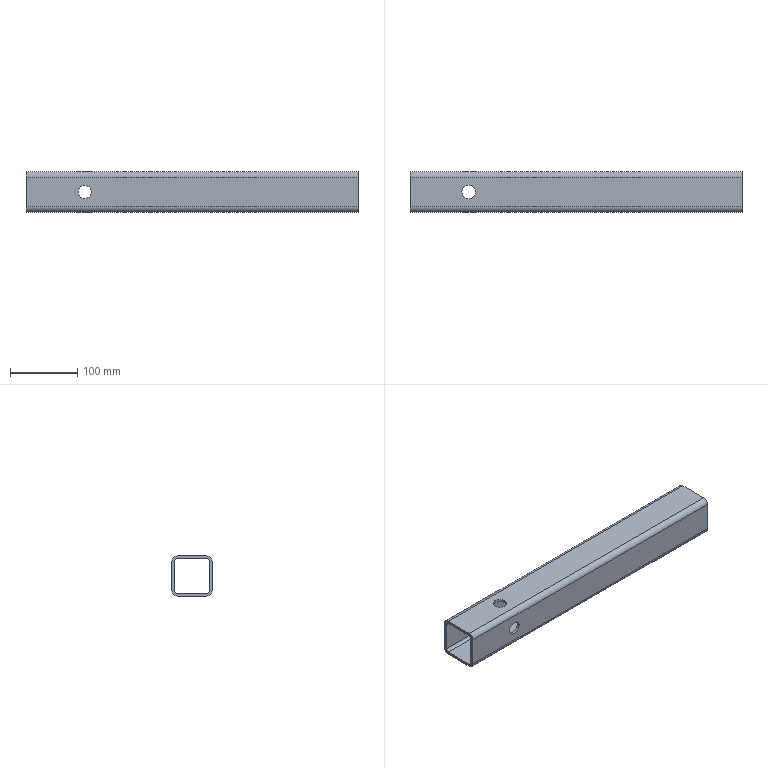Part | SolidWorks | features Cut 2, WeldMemberFeat 1, WeldmentFeature 1 | 1 solid | 26 faces | box 495 x 60 x 60 mm | volume 418098 mm3 | cylinder 16 | plane 10 | commonest cylinder face diameters 20 x8 8 x4 16 x4
STEP:
#1=CARTESIAN_POINT('',(-160.,-30.,10.));
#2=VERTEX_POINT('',#1);
#3=CARTESIAN_POINT('',(-160.,-30.,-10.));
#4=VERTEX_POINT('',#3);
#5=CARTESIAN_POINT('',(-160.,-30.,0.));
#6=DIRECTION('',(0.,-1.,0.));
#7=DIRECTION('',(-1.,0.,0.));
#8=AXIS2_PLACEMENT_3D('',#5,#6,#7);
#9=CIRCLE('',#8,10.);
#10=EDGE_CURVE('',#2,#4,#9,.T.);
#11=ORIENTED_EDGE('',*,*,#10,.T.);
#12=CARTESIAN_POINT('',(-160.,-26.,-10.));
#13=VERTEX_POINT('',#12);
#14=CARTESIAN_POINT('',(-160.,-58.284,-10.));
#15=DIRECTION('',(0.,1.,0.));
#16=VECTOR('',#15,1000.);
#17=LINE('',#14,#16);
#18=EDGE_CURVE('',#4,#13,#17,.T.);
#19=ORIENTED_EDGE('',*,*,#18,.T.);
#20=CARTESIAN_POINT('',(-160.,-26.,10.));
#21=VERTEX_POINT('',#20);
#22=CARTESIAN_POINT('',(-160.,-26.,0.));
#23=DIRECTION('',(0.,1.,0.));
#24=DIRECTION('',(-1.,0.,0.));
#25=AXIS2_PLACEMENT_3D('',#22,#23,#24);
#26=CIRCLE('',#25,10.);
#27=EDGE_CURVE('',#13,#21,#26,.T.);
#28=ORIENTED_EDGE('',*,*,#27,.T.);
#29=CARTESIAN_POINT('',(-160.,-58.284,10.));
#30=DIRECTION('',(0.,1.,0.));
#31=VECTOR('',#30,1000.);
#32=LINE('',#29,#31);
#33=EDGE_CURVE('',#2,#21,#32,.T.);
#34=ORIENTED_EDGE('',*,*,#33,.F.);
#35=EDGE_LOOP('',(#11,#19,#28,#34));
#36=FACE_OUTER_BOUND('',#35,.T.);
#37=CARTESIAN_POINT('',(-160.,-58.284,0.));
#38=DIRECTION('',(0.,1.,0.));
#39=DIRECTION('',(0.,0.,1.));
#40=AXIS2_PLACEMENT_3D('',#37,#38,#39);
#41=CYLINDRICAL_SURFACE('',#40,10.);
#42=ADVANCED_FACE('',(#36),#41,.F.);
#43=CARTESIAN_POINT('',(-160.,26.,10.));
#44=VERTEX_POINT('',#43);
#45=CARTESIAN_POINT('',(-160.,26.,-10.));
#46=VERTEX_POINT('',#45);
#47=CARTESIAN_POINT('',(-160.,26.,0.));
#48=DIRECTION('',(0.,-1.,0.));
#49=DIRECTION('',(1.,0.,0.));
#50=AXIS2_PLACEMENT_3D('',#47,#48,#49);
#51=CIRCLE('',#50,10.);
#52=EDGE_CURVE('',#44,#46,#51,.T.);
#53=ORIENTED_EDGE('',*,*,#52,.T.);
#54=CARTESIAN_POINT('',(-160.,30.,-10.));
#55=VERTEX_POINT('',#54);
#56=CARTESIAN_POINT('',(-160.,-58.284,-10.));
#57=DIRECTION('',(0.,1.,0.));
#58=VECTOR('',#57,1000.);
#59=LINE('',#56,#58);
#60=EDGE_CURVE('',#46,#55,#59,.T.);
#61=ORIENTED_EDGE('',*,*,#60,.T.);
#62=CARTESIAN_POINT('',(-160.,30.,10.));
#63=VERTEX_POINT('',#62);
#64=CARTESIAN_POINT('',(-160.,30.,0.));
#65=DIRECTION('',(0.,1.,0.));
#66=DIRECTION('',(0.,0.,1.));
#67=AXIS2_PLACEMENT_3D('',#64,#65,#66);
#68=CIRCLE('',#67,10.);
#69=EDGE_CURVE('',#55,#63,#68,.T.);
#70=ORIENTED_EDGE('',*,*,#69,.T.);
#71=CARTESIAN_POINT('',(-160.,-58.284,10.));
#72=DIRECTION('',(0.,1.,0.));
#73=VECTOR('',#72,1000.);
#74=LINE('',#71,#73);
#75=EDGE_CURVE('',#44,#63,#74,.T.);
#76=ORIENTED_EDGE('',*,*,#75,.F.);
#77=EDGE_LOOP('',(#53,#61,#70,#76));
#78=FACE_OUTER_BOUND('',#77,.T.);
#79=CARTESIAN_POINT('',(-160.,-58.284,0.));
#80=DIRECTION('',(0.,1.,0.));
#81=DIRECTION('',(0.,0.,1.));
#82=AXIS2_PLACEMENT_3D('',#79,#80,#81);
#83=CYLINDRICAL_SURFACE('',#82,10.);
#84=ADVANCED_FACE('',(#78),#83,.F.);
#85=CARTESIAN_POINT('',(-150.,0.,26.));
#86=VERTEX_POINT('',#85);
#87=CARTESIAN_POINT('',(-170.,0.,26.));
#88=VERTEX_POINT('',#87);
#89=CARTESIAN_POINT('',(-160.,0.,26.));
#90=DIRECTION('',(0.,0.,-1.));
#91=DIRECTION('',(-1.,0.,0.));
#92=AXIS2_PLACEMENT_3D('',#89,#90,#91);
#93=CIRCLE('',#92,10.);
#94=EDGE_CURVE('',#86,#88,#93,.T.);
#95=ORIENTED_EDGE('',*,*,#94,.T.);
#96=CARTESIAN_POINT('',(-170.,0.,30.));
#97=VERTEX_POINT('',#96);
#98=CARTESIAN_POINT('',(-170.,0.,-58.284));
#99=DIRECTION('',(0.,0.,1.));
#100=VECTOR('',#99,1000.);
#101=LINE('',#98,#100);
#102=EDGE_CURVE('',#88,#97,#101,.T.);
#103=ORIENTED_EDGE('',*,*,#102,.T.);
#104=CARTESIAN_POINT('',(-150.,0.,30.));
#105=VERTEX_POINT('',#104);
#106=CARTESIAN_POINT('',(-160.,0.,30.));
#107=DIRECTION('',(0.,0.,1.));
#108=DIRECTION('',(1.,0.,0.));
#109=AXIS2_PLACEMENT_3D('',#106,#107,#108);
#110=CIRCLE('',#109,10.);
#111=EDGE_CURVE('',#97,#105,#110,.T.);
#112=ORIENTED_EDGE('',*,*,#111,.T.);
#113=CARTESIAN_POINT('',(-150.,0.,-58.284));
#114=DIRECTION('',(0.,0.,1.));
#115=VECTOR('',#114,1000.);
#116=LINE('',#113,#115);
#117=EDGE_CURVE('',#86,#105,#116,.T.);
#118=ORIENTED_EDGE('',*,*,#117,.F.);
#119=EDGE_LOOP('',(#95,#103,#112,#118));
#120=FACE_OUTER_BOUND('',#119,.T.);
#121=CARTESIAN_POINT('',(-160.,0.,-58.284));
#122=DIRECTION('',(0.,0.,1.));
#123=DIRECTION('',(1.,0.,0.));
#124=AXIS2_PLACEMENT_3D('',#121,#122,#123);
#125=CYLINDRICAL_SURFACE('',#124,10.);
#126=ADVANCED_FACE('',(#120),#125,.F.);
#127=CARTESIAN_POINT('',(-150.,0.,-30.));
#128=VERTEX_POINT('',#127);
#129=CARTESIAN_POINT('',(-170.,0.,-30.));
#130=VERTEX_POINT('',#129);
#131=CARTESIAN_POINT('',(-160.,0.,-30.));
#132=DIRECTION('',(0.,0.,-1.));
#133=DIRECTION('',(1.,0.,0.));
#134=AXIS2_PLACEMENT_3D('',#131,#132,#133);
#135=CIRCLE('',#134,10.);
#136=EDGE_CURVE('',#128,#130,#135,.T.);
#137=ORIENTED_EDGE('',*,*,#136,.T.);
#138=CARTESIAN_POINT('',(-170.,0.,-26.));
#139=VERTEX_POINT('',#138);
#140=CARTESIAN_POINT('',(-170.,0.,-58.284));
#141=DIRECTION('',(0.,0.,1.));
#142=VECTOR('',#141,1000.);
#143=LINE('',#140,#142);
#144=EDGE_CURVE('',#130,#139,#143,.T.);
#145=ORIENTED_EDGE('',*,*,#144,.T.);
#146=CARTESIAN_POINT('',(-150.,0.,-26.));
#147=VERTEX_POINT('',#146);
#148=CARTESIAN_POINT('',(-160.,0.,-26.));
#149=DIRECTION('',(0.,0.,1.));
#150=DIRECTION('',(1.,0.,0.));
#151=AXIS2_PLACEMENT_3D('',#148,#149,#150);
#152=CIRCLE('',#151,10.);
#153=EDGE_CURVE('',#139,#147,#152,.T.);
#154=ORIENTED_EDGE('',*,*,#153,.T.);
#155=CARTESIAN_POINT('',(-150.,0.,-58.284));
#156=DIRECTION('',(0.,0.,1.));
#157=VECTOR('',#156,1000.);
#158=LINE('',#155,#157);
#159=EDGE_CURVE('',#128,#147,#158,.T.);
#160=ORIENTED_EDGE('',*,*,#159,.F.);
#161=EDGE_LOOP('',(#137,#145,#154,#160));
#162=FACE_OUTER_BOUND('',#161,.T.);
#163=CARTESIAN_POINT('',(-160.,0.,-58.284));
#164=DIRECTION('',(0.,0.,1.));
#165=DIRECTION('',(1.,0.,0.));
#166=AXIS2_PLACEMENT_3D('',#163,#164,#165);
#167=CYLINDRICAL_SURFACE('',#166,10.);
#168=ADVANCED_FACE('',(#162),#167,.F.);
#169=CARTESIAN_POINT('',(-247.5,30.,22.));
#170=VERTEX_POINT('',#169);
#171=CARTESIAN_POINT('',(-247.5,22.,30.));
#172=VERTEX_POINT('',#171);
#173=CARTESIAN_POINT('',(-247.5,22.,22.));
#174=DIRECTION('',(1.,0.,0.));
#175=DIRECTION('',(0.,1.,0.));
#176=AXIS2_PLACEMENT_3D('',#173,#174,#175);
#177=CIRCLE('',#176,8.);
#178=EDGE_CURVE('',#170,#172,#177,.T.);
#179=ORIENTED_EDGE('',*,*,#178,.T.);
#180=CARTESIAN_POINT('',(247.5,22.,30.));
#181=VERTEX_POINT('',#180);
#182=CARTESIAN_POINT('',(247.5,22.,30.));
#183=DIRECTION('',(-1.,0.,0.));
#184=VECTOR('',#183,1000.);
#185=LINE('',#182,#184);
#186=EDGE_CURVE('',#181,#172,#185,.T.);
#187=ORIENTED_EDGE('',*,*,#186,.F.);
#188=CARTESIAN_POINT('',(247.5,30.,22.));
#189=VERTEX_POINT('',#188);
#190=CARTESIAN_POINT('',(247.5,22.,22.));
#191=DIRECTION('',(1.,0.,0.));
#192=DIRECTION('',(0.,1.,0.));
#193=AXIS2_PLACEMENT_3D('',#190,#191,#192);
#194=CIRCLE('',#193,8.);
#195=EDGE_CURVE('',#189,#181,#194,.T.);
#196=ORIENTED_EDGE('',*,*,#195,.F.);
#197=CARTESIAN_POINT('',(247.5,30.,22.));
#198=DIRECTION('',(-1.,0.,0.));
#199=VECTOR('',#198,1000.);
#200=LINE('',#197,#199);
#201=EDGE_CURVE('',#189,#170,#200,.T.);
#202=ORIENTED_EDGE('',*,*,#201,.T.);
#203=EDGE_LOOP('',(#179,#187,#196,#202));
#204=FACE_OUTER_BOUND('',#203,.T.);
#205=CARTESIAN_POINT('',(247.5,22.,22.));
#206=DIRECTION('',(-1.,0.,0.));
#207=DIRECTION('',(0.,-1.,0.));
#208=AXIS2_PLACEMENT_3D('',#205,#206,#207);
#209=CYLINDRICAL_SURFACE('',#208,8.);
#210=ADVANCED_FACE('',(#204),#209,.T.);
#211=CARTESIAN_POINT('',(-160.,0.,30.));
#212=DIRECTION('',(0.,0.,1.));
#213=DIRECTION('',(1.,0.,0.));
#214=AXIS2_PLACEMENT_3D('',#211,#212,#213);
#215=CIRCLE('',#214,10.);
#216=EDGE_CURVE('',#105,#97,#215,.T.);
#217=ORIENTED_EDGE('',*,*,#216,.F.);
#218=ORIENTED_EDGE('',*,*,#111,.F.);
#219=EDGE_LOOP('',(#217,#218));
#220=FACE_BOUND('',#219,.T.);
#221=CARTESIAN_POINT('',(-247.5,-22.,30.));
#222=VERTEX_POINT('',#221);
#223=CARTESIAN_POINT('',(-247.5,22.,30.));
#224=DIRECTION('',(0.,-1.,0.));
#225=VECTOR('',#224,1000.);
#226=LINE('',#223,#225);
#227=EDGE_CURVE('',#172,#222,#226,.T.);
#228=ORIENTED_EDGE('',*,*,#227,.T.);
#229=CARTESIAN_POINT('',(247.5,-22.,30.));
#230=VERTEX_POINT('',#229);
#231=CARTESIAN_POINT('',(247.5,-22.,30.));
#232=DIRECTION('',(-1.,0.,0.));
#233=VECTOR('',#232,1000.);
#234=LINE('',#231,#233);
#235=EDGE_CURVE('',#230,#222,#234,.T.);
#236=ORIENTED_EDGE('',*,*,#235,.F.);
#237=CARTESIAN_POINT('',(247.5,22.,30.));
#238=DIRECTION('',(0.,-1.,0.));
#239=VECTOR('',#238,1000.);
#240=LINE('',#237,#239);
#241=EDGE_CURVE('',#181,#230,#240,.T.);
#242=ORIENTED_EDGE('',*,*,#241,.F.);
#243=ORIENTED_EDGE('',*,*,#186,.T.);
#244=EDGE_LOOP('',(#228,#236,#242,#243));
#245=FACE_OUTER_BOUND('',#244,.T.);
#246=CARTESIAN_POINT('',(247.5,22.,30.));
#247=DIRECTION('',(0.,0.,-1.));
#248=DIRECTION('',(-1.,0.,0.));
#249=AXIS2_PLACEMENT_3D('',#246,#247,#248);
#250=PLANE('',#249);
#251=ADVANCED_FACE('',(#220,#245),#250,.F.);
#252=CARTESIAN_POINT('',(-247.5,-30.,22.));
#253=VERTEX_POINT('',#252);
#254=CARTESIAN_POINT('',(-247.5,-22.,22.));
#255=DIRECTION('',(1.,0.,0.));
#256=DIRECTION('',(0.,1.,0.));
#257=AXIS2_PLACEMENT_3D('',#254,#255,#256);
#258=CIRCLE('',#257,8.);
#259=EDGE_CURVE('',#222,#253,#258,.T.);
#260=ORIENTED_EDGE('',*,*,#259,.T.);
#261=CARTESIAN_POINT('',(247.5,-30.,22.));
#262=VERTEX_POINT('',#261);
#263=CARTESIAN_POINT('',(247.5,-30.,22.));
#264=DIRECTION('',(-1.,0.,0.));
#265=VECTOR('',#264,1000.);
#266=LINE('',#263,#265);
#267=EDGE_CURVE('',#262,#253,#266,.T.);
#268=ORIENTED_EDGE('',*,*,#267,.F.);
#269=CARTESIAN_POINT('',(247.5,-22.,22.));
#270=DIRECTION('',(1.,0.,0.));
#271=DIRECTION('',(0.,1.,0.));
#272=AXIS2_PLACEMENT_3D('',#269,#270,#271);
#273=CIRCLE('',#272,8.);
#274=EDGE_CURVE('',#230,#262,#273,.T.);
#275=ORIENTED_EDGE('',*,*,#274,.F.);
#276=ORIENTED_EDGE('',*,*,#235,.T.);
#277=EDGE_LOOP('',(#260,#268,#275,#276));
#278=FACE_OUTER_BOUND('',#277,.T.);
#279=CARTESIAN_POINT('',(247.5,-22.,22.));
#280=DIRECTION('',(-1.,0.,0.));
#281=DIRECTION('',(0.,-1.,0.));
#282=AXIS2_PLACEMENT_3D('',#279,#280,#281);
#283=CYLINDRICAL_SURFACE('',#282,8.);
#284=ADVANCED_FACE('',(#278),#283,.T.);
#285=ORIENTED_EDGE('',*,*,#10,.F.);
#286=CARTESIAN_POINT('',(-160.,-30.,0.));
#287=DIRECTION('',(0.,-1.,0.));
#288=DIRECTION('',(-1.,0.,0.));
#289=AXIS2_PLACEMENT_3D('',#286,#287,#288);
#290=CIRCLE('',#289,10.);
#291=EDGE_CURVE('',#4,#2,#290,.T.);
#292=ORIENTED_EDGE('',*,*,#291,.F.);
#293=EDGE_LOOP('',(#285,#292));
#294=FACE_BOUND('',#293,.T.);
#295=CARTESIAN_POINT('',(-247.5,-30.,-22.));
#296=VERTEX_POINT('',#295);
#297=CARTESIAN_POINT('',(-247.5,-30.,-22.));
#298=DIRECTION('',(0.,0.,-1.));
#299=VECTOR('',#298,1000.);
#300=LINE('',#297,#299);
#301=EDGE_CURVE('',#253,#296,#300,.T.);
#302=ORIENTED_EDGE('',*,*,#301,.T.);
#303=CARTESIAN_POINT('',(247.5,-30.,-22.));
#304=VERTEX_POINT('',#303);
#305=CARTESIAN_POINT('',(247.5,-30.,-22.));
#306=DIRECTION('',(-1.,0.,0.));
#307=VECTOR('',#306,1000.);
#308=LINE('',#305,#307);
#309=EDGE_CURVE('',#304,#296,#308,.T.);
#310=ORIENTED_EDGE('',*,*,#309,.F.);
#311=CARTESIAN_POINT('',(247.5,-30.,-22.));
#312=DIRECTION('',(0.,0.,-1.));
#313=VECTOR('',#312,1000.);
#314=LINE('',#311,#313);
#315=EDGE_CURVE('',#262,#304,#314,.T.);
#316=ORIENTED_EDGE('',*,*,#315,.F.);
#317=ORIENTED_EDGE('',*,*,#267,.T.);
#318=EDGE_LOOP('',(#302,#310,#316,#317));
#319=FACE_OUTER_BOUND('',#318,.T.);
#320=CARTESIAN_POINT('',(247.5,-30.,-22.));
#321=DIRECTION('',(0.,1.,0.));
#322=DIRECTION('',(-1.,0.,0.));
#323=AXIS2_PLACEMENT_3D('',#320,#321,#322);
#324=PLANE('',#323);
#325=ADVANCED_FACE('',(#294,#319),#324,.F.);
#326=CARTESIAN_POINT('',(-247.5,-22.,-30.));
#327=VERTEX_POINT('',#326);
#328=CARTESIAN_POINT('',(-247.5,-22.,-22.));
#329=DIRECTION('',(1.,0.,0.));
#330=DIRECTION('',(0.,1.,0.));
#331=AXIS2_PLACEMENT_3D('',#328,#329,#330);
#332=CIRCLE('',#331,8.);
#333=EDGE_CURVE('',#296,#327,#332,.T.);
#334=ORIENTED_EDGE('',*,*,#333,.T.);
#335=CARTESIAN_POINT('',(247.5,-22.,-30.));
#336=VERTEX_POINT('',#335);
#337=CARTESIAN_POINT('',(247.5,-22.,-30.));
#338=DIRECTION('',(-1.,0.,0.));
#339=VECTOR('',#338,1000.);
#340=LINE('',#337,#339);
#341=EDGE_CURVE('',#336,#327,#340,.T.);
#342=ORIENTED_EDGE('',*,*,#341,.F.);
#343=CARTESIAN_POINT('',(247.5,-22.,-22.));
#344=DIRECTION('',(1.,0.,0.));
#345=DIRECTION('',(0.,1.,0.));
#346=AXIS2_PLACEMENT_3D('',#343,#344,#345);
#347=CIRCLE('',#346,8.);
#348=EDGE_CURVE('',#304,#336,#347,.T.);
#349=ORIENTED_EDGE('',*,*,#348,.F.);
#350=ORIENTED_EDGE('',*,*,#309,.T.);
#351=EDGE_LOOP('',(#334,#342,#349,#350));
#352=FACE_OUTER_BOUND('',#351,.T.);
#353=CARTESIAN_POINT('',(247.5,-22.,-22.));
#354=DIRECTION('',(-1.,0.,0.));
#355=DIRECTION('',(0.,-1.,0.));
#356=AXIS2_PLACEMENT_3D('',#353,#354,#355);
#357=CYLINDRICAL_SURFACE('',#356,8.);
#358=ADVANCED_FACE('',(#352),#357,.T.);
#359=ORIENTED_EDGE('',*,*,#136,.F.);
#360=CARTESIAN_POINT('',(-160.,0.,-30.));
#361=DIRECTION('',(0.,0.,-1.));
#362=DIRECTION('',(1.,0.,0.));
#363=AXIS2_PLACEMENT_3D('',#360,#361,#362);
#364=CIRCLE('',#363,10.);
#365=EDGE_CURVE('',#130,#128,#364,.T.);
#366=ORIENTED_EDGE('',*,*,#365,.F.);
#367=EDGE_LOOP('',(#359,#366));
#368=FACE_BOUND('',#367,.T.);
#369=CARTESIAN_POINT('',(-247.5,22.,-30.));
#370=VERTEX_POINT('',#369);
#371=CARTESIAN_POINT('',(-247.5,-22.,-30.));
#372=DIRECTION('',(0.,1.,0.));
#373=VECTOR('',#372,1000.);
#374=LINE('',#371,#373);
#375=EDGE_CURVE('',#327,#370,#374,.T.);
#376=ORIENTED_EDGE('',*,*,#375,.T.);
#377=CARTESIAN_POINT('',(247.5,22.,-30.));
#378=VERTEX_POINT('',#377);
#379=CARTESIAN_POINT('',(247.5,22.,-30.));
#380=DIRECTION('',(-1.,0.,0.));
#381=VECTOR('',#380,1000.);
#382=LINE('',#379,#381);
#383=EDGE_CURVE('',#378,#370,#382,.T.);
#384=ORIENTED_EDGE('',*,*,#383,.F.);
#385=CARTESIAN_POINT('',(247.5,-22.,-30.));
#386=DIRECTION('',(0.,1.,0.));
#387=VECTOR('',#386,1000.);
#388=LINE('',#385,#387);
#389=EDGE_CURVE('',#336,#378,#388,.T.);
#390=ORIENTED_EDGE('',*,*,#389,.F.);
#391=ORIENTED_EDGE('',*,*,#341,.T.);
#392=EDGE_LOOP('',(#376,#384,#390,#391));
#393=FACE_OUTER_BOUND('',#392,.T.);
#394=CARTESIAN_POINT('',(247.5,-22.,-30.));
#395=DIRECTION('',(0.,0.,1.));
#396=DIRECTION('',(1.,0.,0.));
#397=AXIS2_PLACEMENT_3D('',#394,#395,#396);
#398=PLANE('',#397);
#399=ADVANCED_FACE('',(#368,#393),#398,.F.);
#400=CARTESIAN_POINT('',(-247.5,30.,-22.));
#401=VERTEX_POINT('',#400);
#402=CARTESIAN_POINT('',(-247.5,22.,-22.));
#403=DIRECTION('',(1.,0.,0.));
#404=DIRECTION('',(0.,1.,0.));
#405=AXIS2_PLACEMENT_3D('',#402,#403,#404);
#406=CIRCLE('',#405,8.);
#407=EDGE_CURVE('',#370,#401,#406,.T.);
#408=ORIENTED_EDGE('',*,*,#407,.T.);
#409=CARTESIAN_POINT('',(247.5,30.,-22.));
#410=VERTEX_POINT('',#409);
#411=CARTESIAN_POINT('',(247.5,30.,-22.));
#412=DIRECTION('',(-1.,0.,0.));
#413=VECTOR('',#412,1000.);
#414=LINE('',#411,#413);
#415=EDGE_CURVE('',#410,#401,#414,.T.);
#416=ORIENTED_EDGE('',*,*,#415,.F.);
#417=CARTESIAN_POINT('',(247.5,22.,-22.));
#418=DIRECTION('',(1.,0.,0.));
#419=DIRECTION('',(0.,1.,0.));
#420=AXIS2_PLACEMENT_3D('',#417,#418,#419);
#421=CIRCLE('',#420,8.);
#422=EDGE_CURVE('',#378,#410,#421,.T.);
#423=ORIENTED_EDGE('',*,*,#422,.F.);
#424=ORIENTED_EDGE('',*,*,#383,.T.);
#425=EDGE_LOOP('',(#408,#416,#423,#424));
#426=FACE_OUTER_BOUND('',#425,.T.);
#427=CARTESIAN_POINT('',(247.5,22.,-22.));
#428=DIRECTION('',(-1.,0.,0.));
#429=DIRECTION('',(0.,-1.,0.));
#430=AXIS2_PLACEMENT_3D('',#427,#428,#429);
#431=CYLINDRICAL_SURFACE('',#430,8.);
#432=ADVANCED_FACE('',(#426),#431,.T.);
#433=CARTESIAN_POINT('',(-247.5,-22.,26.));
#434=VERTEX_POINT('',#433);
#435=CARTESIAN_POINT('',(-247.5,-26.,22.));
#436=VERTEX_POINT('',#435);
#437=CARTESIAN_POINT('',(-247.5,-22.,22.));
#438=DIRECTION('',(1.,0.,0.));
#439=DIRECTION('',(0.,1.,0.));
#440=AXIS2_PLACEMENT_3D('',#437,#438,#439);
#441=CIRCLE('',#440,4.);
#442=EDGE_CURVE('',#434,#436,#441,.T.);
#443=ORIENTED_EDGE('',*,*,#442,.F.);
#444=CARTESIAN_POINT('',(247.5,-22.,26.));
#445=VERTEX_POINT('',#444);
#446=CARTESIAN_POINT('',(247.5,-22.,26.));
#447=DIRECTION('',(-1.,0.,0.));
#448=VECTOR('',#447,1000.);
#449=LINE('',#446,#448);
#450=EDGE_CURVE('',#445,#434,#449,.T.);
#451=ORIENTED_EDGE('',*,*,#450,.F.);
#452=CARTESIAN_POINT('',(247.5,-26.,22.));
#453=VERTEX_POINT('',#452);
#454=CARTESIAN_POINT('',(247.5,-22.,22.));
#455=DIRECTION('',(1.,0.,0.));
#456=DIRECTION('',(0.,1.,0.));
#457=AXIS2_PLACEMENT_3D('',#454,#455,#456);
#458=CIRCLE('',#457,4.);
#459=EDGE_CURVE('',#445,#453,#458,.T.);
#460=ORIENTED_EDGE('',*,*,#459,.T.);
#461=CARTESIAN_POINT('',(247.5,-26.,22.));
#462=DIRECTION('',(-1.,0.,0.));
#463=VECTOR('',#462,1000.);
#464=LINE('',#461,#463);
#465=EDGE_CURVE('',#453,#436,#464,.T.);
#466=ORIENTED_EDGE('',*,*,#465,.T.);
#467=EDGE_LOOP('',(#443,#451,#460,#466));
#468=FACE_OUTER_BOUND('',#467,.T.);
#469=CARTESIAN_POINT('',(247.5,-22.,22.));
#470=DIRECTION('',(-1.,0.,0.));
#471=DIRECTION('',(0.,-1.,0.));
#472=AXIS2_PLACEMENT_3D('',#469,#470,#471);
#473=CYLINDRICAL_SURFACE('',#472,4.);
#474=ADVANCED_FACE('',(#468),#473,.F.);
#475=ORIENTED_EDGE('',*,*,#94,.F.);
#476=CARTESIAN_POINT('',(-160.,0.,26.));
#477=DIRECTION('',(0.,0.,-1.));
#478=DIRECTION('',(-1.,0.,0.));
#479=AXIS2_PLACEMENT_3D('',#476,#477,#478);
#480=CIRCLE('',#479,10.);
#481=EDGE_CURVE('',#88,#86,#480,.T.);
#482=ORIENTED_EDGE('',*,*,#481,.F.);
#483=EDGE_LOOP('',(#475,#482));
#484=FACE_BOUND('',#483,.T.);
#485=CARTESIAN_POINT('',(-247.5,22.,26.));
#486=VERTEX_POINT('',#485);
#487=CARTESIAN_POINT('',(-247.5,22.,26.));
#488=DIRECTION('',(0.,-1.,0.));
#489=VECTOR('',#488,1000.);
#490=LINE('',#487,#489);
#491=EDGE_CURVE('',#486,#434,#490,.T.);
#492=ORIENTED_EDGE('',*,*,#491,.F.);
#493=CARTESIAN_POINT('',(247.5,22.,26.));
#494=VERTEX_POINT('',#493);
#495=CARTESIAN_POINT('',(247.5,22.,26.));
#496=DIRECTION('',(-1.,0.,0.));
#497=VECTOR('',#496,1000.);
#498=LINE('',#495,#497);
#499=EDGE_CURVE('',#494,#486,#498,.T.);
#500=ORIENTED_EDGE('',*,*,#499,.F.);
#501=CARTESIAN_POINT('',(247.5,22.,26.));
#502=DIRECTION('',(0.,-1.,0.));
#503=VECTOR('',#502,1000.);
#504=LINE('',#501,#503);
#505=EDGE_CURVE('',#494,#445,#504,.T.);
#506=ORIENTED_EDGE('',*,*,#505,.T.);
#507=ORIENTED_EDGE('',*,*,#450,.T.);
#508=EDGE_LOOP('',(#492,#500,#506,#507));
#509=FACE_OUTER_BOUND('',#508,.T.);
#510=CARTESIAN_POINT('',(247.5,22.,26.));
#511=DIRECTION('',(0.,0.,-1.));
#512=DIRECTION('',(-1.,0.,0.));
#513=AXIS2_PLACEMENT_3D('',#510,#511,#512);
#514=PLANE('',#513);
#515=ADVANCED_FACE('',(#484,#509),#514,.T.);
#516=CARTESIAN_POINT('',(-247.5,26.,22.));
#517=VERTEX_POINT('',#516);
#518=CARTESIAN_POINT('',(-247.5,22.,22.));
#519=DIRECTION('',(1.,0.,0.));
#520=DIRECTION('',(0.,1.,0.));
#521=AXIS2_PLACEMENT_3D('',#518,#519,#520);
#522=CIRCLE('',#521,4.);
#523=EDGE_CURVE('',#517,#486,#522,.T.);
#524=ORIENTED_EDGE('',*,*,#523,.F.);
#525=CARTESIAN_POINT('',(247.5,26.,22.));
#526=VERTEX_POINT('',#525);
#527=CARTESIAN_POINT('',(247.5,26.,22.));
#528=DIRECTION('',(-1.,0.,0.));
#529=VECTOR('',#528,1000.);
#530=LINE('',#527,#529);
#531=EDGE_CURVE('',#526,#517,#530,.T.);
#532=ORIENTED_EDGE('',*,*,#531,.F.);
#533=CARTESIAN_POINT('',(247.5,22.,22.));
#534=DIRECTION('',(1.,0.,0.));
#535=DIRECTION('',(0.,1.,0.));
#536=AXIS2_PLACEMENT_3D('',#533,#534,#535);
#537=CIRCLE('',#536,4.);
#538=EDGE_CURVE('',#526,#494,#537,.T.);
#539=ORIENTED_EDGE('',*,*,#538,.T.);
#540=ORIENTED_EDGE('',*,*,#499,.T.);
#541=EDGE_LOOP('',(#524,#532,#539,#540));
#542=FACE_OUTER_BOUND('',#541,.T.);
#543=CARTESIAN_POINT('',(247.5,22.,22.));
#544=DIRECTION('',(-1.,0.,0.));
#545=DIRECTION('',(0.,-1.,0.));
#546=AXIS2_PLACEMENT_3D('',#543,#544,#545);
#547=CYLINDRICAL_SURFACE('',#546,4.);
#548=ADVANCED_FACE('',(#542),#547,.F.);
#549=ORIENTED_EDGE('',*,*,#52,.F.);
#550=CARTESIAN_POINT('',(-160.,26.,0.));
#551=DIRECTION('',(0.,-1.,0.));
#552=DIRECTION('',(1.,0.,0.));
#553=AXIS2_PLACEMENT_3D('',#550,#551,#552);
#554=CIRCLE('',#553,10.);
#555=EDGE_CURVE('',#46,#44,#554,.T.);
#556=ORIENTED_EDGE('',*,*,#555,.F.);
#557=EDGE_LOOP('',(#549,#556));
#558=FACE_BOUND('',#557,.T.);
#559=CARTESIAN_POINT('',(-247.5,26.,-22.));
#560=VERTEX_POINT('',#559);
#561=CARTESIAN_POINT('',(-247.5,26.,22.));
#562=DIRECTION('',(0.,0.,1.));
#563=VECTOR('',#562,1000.);
#564=LINE('',#561,#563);
#565=EDGE_CURVE('',#560,#517,#564,.T.);
#566=ORIENTED_EDGE('',*,*,#565,.F.);
#567=CARTESIAN_POINT('',(247.5,26.,-22.));
#568=VERTEX_POINT('',#567);
#569=CARTESIAN_POINT('',(247.5,26.,-22.));
#570=DIRECTION('',(-1.,0.,0.));
#571=VECTOR('',#570,1000.);
#572=LINE('',#569,#571);
#573=EDGE_CURVE('',#568,#560,#572,.T.);
#574=ORIENTED_EDGE('',*,*,#573,.F.);
#575=CARTESIAN_POINT('',(247.5,26.,22.));
#576=DIRECTION('',(0.,0.,1.));
#577=VECTOR('',#576,1000.);
#578=LINE('',#575,#577);
#579=EDGE_CURVE('',#568,#526,#578,.T.);
#580=ORIENTED_EDGE('',*,*,#579,.T.);
#581=ORIENTED_EDGE('',*,*,#531,.T.);
#582=EDGE_LOOP('',(#566,#574,#580,#581));
#583=FACE_OUTER_BOUND('',#582,.T.);
#584=CARTESIAN_POINT('',(247.5,26.,22.));
#585=DIRECTION('',(0.,-1.,0.));
#586=DIRECTION('',(1.,0.,0.));
#587=AXIS2_PLACEMENT_3D('',#584,#585,#586);
#588=PLANE('',#587);
#589=ADVANCED_FACE('',(#558,#583),#588,.T.);
#590=CARTESIAN_POINT('',(-247.5,22.,-26.));
#591=VERTEX_POINT('',#590);
#592=CARTESIAN_POINT('',(-247.5,22.,-22.));
#593=DIRECTION('',(1.,0.,0.));
#594=DIRECTION('',(0.,1.,0.));
#595=AXIS2_PLACEMENT_3D('',#592,#593,#594);
#596=CIRCLE('',#595,4.);
#597=EDGE_CURVE('',#591,#560,#596,.T.);
#598=ORIENTED_EDGE('',*,*,#597,.F.);
#599=CARTESIAN_POINT('',(247.5,22.,-26.));
#600=VERTEX_POINT('',#599);
#601=CARTESIAN_POINT('',(247.5,22.,-26.));
#602=DIRECTION('',(-1.,0.,0.));
#603=VECTOR('',#602,1000.);
#604=LINE('',#601,#603);
#605=EDGE_CURVE('',#600,#591,#604,.T.);
#606=ORIENTED_EDGE('',*,*,#605,.F.);
#607=CARTESIAN_POINT('',(247.5,22.,-22.));
#608=DIRECTION('',(1.,0.,0.));
#609=DIRECTION('',(0.,1.,0.));
#610=AXIS2_PLACEMENT_3D('',#607,#608,#609);
#611=CIRCLE('',#610,4.);
#612=EDGE_CURVE('',#600,#568,#611,.T.);
#613=ORIENTED_EDGE('',*,*,#612,.T.);
#614=ORIENTED_EDGE('',*,*,#573,.T.);
#615=EDGE_LOOP('',(#598,#606,#613,#614));
#616=FACE_OUTER_BOUND('',#615,.T.);
#617=CARTESIAN_POINT('',(247.5,22.,-22.));
#618=DIRECTION('',(-1.,0.,0.));
#619=DIRECTION('',(0.,-1.,0.));
#620=AXIS2_PLACEMENT_3D('',#617,#618,#619);
#621=CYLINDRICAL_SURFACE('',#620,4.);
#622=ADVANCED_FACE('',(#616),#621,.F.);
#623=CARTESIAN_POINT('',(-160.,0.,-26.));
#624=DIRECTION('',(0.,0.,1.));
#625=DIRECTION('',(1.,0.,0.));
#626=AXIS2_PLACEMENT_3D('',#623,#624,#625);
#627=CIRCLE('',#626,10.);
#628=EDGE_CURVE('',#147,#139,#627,.T.);
#629=ORIENTED_EDGE('',*,*,#628,.F.);
#630=ORIENTED_EDGE('',*,*,#153,.F.);
#631=EDGE_LOOP('',(#629,#630));
#632=FACE_BOUND('',#631,.T.);
#633=CARTESIAN_POINT('',(-247.5,-22.,-26.));
#634=VERTEX_POINT('',#633);
#635=CARTESIAN_POINT('',(-247.5,-22.,-26.));
#636=DIRECTION('',(0.,1.,0.));
#637=VECTOR('',#636,1000.);
#638=LINE('',#635,#637);
#639=EDGE_CURVE('',#634,#591,#638,.T.);
#640=ORIENTED_EDGE('',*,*,#639,.F.);
#641=CARTESIAN_POINT('',(247.5,-22.,-26.));
#642=VERTEX_POINT('',#641);
#643=CARTESIAN_POINT('',(247.5,-22.,-26.));
#644=DIRECTION('',(-1.,0.,0.));
#645=VECTOR('',#644,1000.);
#646=LINE('',#643,#645);
#647=EDGE_CURVE('',#642,#634,#646,.T.);
#648=ORIENTED_EDGE('',*,*,#647,.F.);
#649=CARTESIAN_POINT('',(247.5,-22.,-26.));
#650=DIRECTION('',(0.,1.,0.));
#651=VECTOR('',#650,1000.);
#652=LINE('',#649,#651);
#653=EDGE_CURVE('',#642,#600,#652,.T.);
#654=ORIENTED_EDGE('',*,*,#653,.T.);
#655=ORIENTED_EDGE('',*,*,#605,.T.);
#656=EDGE_LOOP('',(#640,#648,#654,#655));
#657=FACE_OUTER_BOUND('',#656,.T.);
#658=CARTESIAN_POINT('',(247.5,-22.,-26.));
#659=DIRECTION('',(0.,0.,1.));
#660=DIRECTION('',(1.,0.,0.));
#661=AXIS2_PLACEMENT_3D('',#658,#659,#660);
#662=PLANE('',#661);
#663=ADVANCED_FACE('',(#632,#657),#662,.T.);
#664=CARTESIAN_POINT('',(-247.5,-26.,-22.));
#665=VERTEX_POINT('',#664);
#666=CARTESIAN_POINT('',(-247.5,-22.,-22.));
#667=DIRECTION('',(1.,0.,0.));
#668=DIRECTION('',(0.,1.,0.));
#669=AXIS2_PLACEMENT_3D('',#666,#667,#668);
#670=CIRCLE('',#669,4.);
#671=EDGE_CURVE('',#665,#634,#670,.T.);
#672=ORIENTED_EDGE('',*,*,#671,.F.);
#673=CARTESIAN_POINT('',(247.5,-26.,-22.));
#674=VERTEX_POINT('',#673);
#675=CARTESIAN_POINT('',(247.5,-26.,-22.));
#676=DIRECTION('',(-1.,0.,0.));
#677=VECTOR('',#676,1000.);
#678=LINE('',#675,#677);
#679=EDGE_CURVE('',#674,#665,#678,.T.);
#680=ORIENTED_EDGE('',*,*,#679,.F.);
#681=CARTESIAN_POINT('',(247.5,-22.,-22.));
#682=DIRECTION('',(1.,0.,0.));
#683=DIRECTION('',(0.,1.,0.));
#684=AXIS2_PLACEMENT_3D('',#681,#682,#683);
#685=CIRCLE('',#684,4.);
#686=EDGE_CURVE('',#674,#642,#685,.T.);
#687=ORIENTED_EDGE('',*,*,#686,.T.);
#688=ORIENTED_EDGE('',*,*,#647,.T.);
#689=EDGE_LOOP('',(#672,#680,#687,#688));
#690=FACE_OUTER_BOUND('',#689,.T.);
#691=CARTESIAN_POINT('',(247.5,-22.,-22.));
#692=DIRECTION('',(-1.,0.,0.));
#693=DIRECTION('',(0.,-1.,0.));
#694=AXIS2_PLACEMENT_3D('',#691,#692,#693);
#695=CYLINDRICAL_SURFACE('',#694,4.);
#696=ADVANCED_FACE('',(#690),#695,.F.);
#697=CARTESIAN_POINT('',(-160.,-26.,0.));
#698=DIRECTION('',(0.,1.,0.));
#699=DIRECTION('',(-1.,0.,0.));
#700=AXIS2_PLACEMENT_3D('',#697,#698,#699);
#701=CIRCLE('',#700,10.);
#702=EDGE_CURVE('',#21,#13,#701,.T.);
#703=ORIENTED_EDGE('',*,*,#702,.F.);
#704=ORIENTED_EDGE('',*,*,#27,.F.);
#705=EDGE_LOOP('',(#703,#704));
#706=FACE_BOUND('',#705,.T.);
#707=CARTESIAN_POINT('',(-247.5,-26.,-22.));
#708=DIRECTION('',(0.,0.,-1.));
#709=VECTOR('',#708,1000.);
#710=LINE('',#707,#709);
#711=EDGE_CURVE('',#436,#665,#710,.T.);
#712=ORIENTED_EDGE('',*,*,#711,.F.);
#713=ORIENTED_EDGE('',*,*,#465,.F.);
#714=CARTESIAN_POINT('',(247.5,-26.,-22.));
#715=DIRECTION('',(0.,0.,-1.));
#716=VECTOR('',#715,1000.);
#717=LINE('',#714,#716);
#718=EDGE_CURVE('',#453,#674,#717,.T.);
#719=ORIENTED_EDGE('',*,*,#718,.T.);
#720=ORIENTED_EDGE('',*,*,#679,.T.);
#721=EDGE_LOOP('',(#712,#713,#719,#720));
#722=FACE_OUTER_BOUND('',#721,.T.);
#723=CARTESIAN_POINT('',(247.5,-26.,-22.));
#724=DIRECTION('',(0.,1.,0.));
#725=DIRECTION('',(-1.,0.,0.));
#726=AXIS2_PLACEMENT_3D('',#723,#724,#725);
#727=PLANE('',#726);
#728=ADVANCED_FACE('',(#706,#722),#727,.T.);
#729=CARTESIAN_POINT('',(-160.,30.,0.));
#730=DIRECTION('',(0.,1.,0.));
#731=DIRECTION('',(0.,0.,1.));
#732=AXIS2_PLACEMENT_3D('',#729,#730,#731);
#733=CIRCLE('',#732,10.);
#734=EDGE_CURVE('',#63,#55,#733,.T.);
#735=ORIENTED_EDGE('',*,*,#734,.F.);
#736=ORIENTED_EDGE('',*,*,#69,.F.);
#737=EDGE_LOOP('',(#735,#736));
#738=FACE_BOUND('',#737,.T.);
#739=CARTESIAN_POINT('',(-247.5,30.,22.));
#740=DIRECTION('',(0.,0.,1.));
#741=VECTOR('',#740,1000.);
#742=LINE('',#739,#741);
#743=EDGE_CURVE('',#401,#170,#742,.T.);
#744=ORIENTED_EDGE('',*,*,#743,.T.);
#745=ORIENTED_EDGE('',*,*,#201,.F.);
#746=CARTESIAN_POINT('',(247.5,30.,22.));
#747=DIRECTION('',(0.,0.,1.));
#748=VECTOR('',#747,1000.);
#749=LINE('',#746,#748);
#750=EDGE_CURVE('',#410,#189,#749,.T.);
#751=ORIENTED_EDGE('',*,*,#750,.F.);
#752=ORIENTED_EDGE('',*,*,#415,.T.);
#753=EDGE_LOOP('',(#744,#745,#751,#752));
#754=FACE_OUTER_BOUND('',#753,.T.);
#755=CARTESIAN_POINT('',(247.5,30.,22.));
#756=DIRECTION('',(0.,-1.,0.));
#757=DIRECTION('',(1.,0.,0.));
#758=AXIS2_PLACEMENT_3D('',#755,#756,#757);
#759=PLANE('',#758);
#760=ADVANCED_FACE('',(#738,#754),#759,.F.);
#761=ORIENTED_EDGE('',*,*,#459,.F.);
#762=ORIENTED_EDGE('',*,*,#505,.F.);
#763=ORIENTED_EDGE('',*,*,#538,.F.);
#764=ORIENTED_EDGE('',*,*,#579,.F.);
#765=ORIENTED_EDGE('',*,*,#612,.F.);
#766=ORIENTED_EDGE('',*,*,#653,.F.);
#767=ORIENTED_EDGE('',*,*,#686,.F.);
#768=ORIENTED_EDGE('',*,*,#718,.F.);
#769=EDGE_LOOP('',(#761,#762,#763,#764,#765,#766,#767,#768));
#770=FACE_BOUND('',#769,.T.);
#771=ORIENTED_EDGE('',*,*,#195,.T.);
#772=ORIENTED_EDGE('',*,*,#241,.T.);
#773=ORIENTED_EDGE('',*,*,#274,.T.);
#774=ORIENTED_EDGE('',*,*,#315,.T.);
#775=ORIENTED_EDGE('',*,*,#348,.T.);
#776=ORIENTED_EDGE('',*,*,#389,.T.);
#777=ORIENTED_EDGE('',*,*,#422,.T.);
#778=ORIENTED_EDGE('',*,*,#750,.T.);
#779=EDGE_LOOP('',(#771,#772,#773,#774,#775,#776,#777,#778));
#780=FACE_OUTER_BOUND('',#779,.T.);
#781=CARTESIAN_POINT('',(247.5,22.,22.));
#782=DIRECTION('',(1.,0.,0.));
#783=DIRECTION('',(0.,1.,0.));
#784=AXIS2_PLACEMENT_3D('',#781,#782,#783);
#785=PLANE('',#784);
#786=ADVANCED_FACE('',(#770,#780),#785,.T.);
#787=ORIENTED_EDGE('',*,*,#442,.T.);
#788=ORIENTED_EDGE('',*,*,#711,.T.);
#789=ORIENTED_EDGE('',*,*,#671,.T.);
#790=ORIENTED_EDGE('',*,*,#639,.T.);
#791=ORIENTED_EDGE('',*,*,#597,.T.);
#792=ORIENTED_EDGE('',*,*,#565,.T.);
#793=ORIENTED_EDGE('',*,*,#523,.T.);
#794=ORIENTED_EDGE('',*,*,#491,.T.);
#795=EDGE_LOOP('',(#787,#788,#789,#790,#791,#792,#793,#794));
#796=FACE_BOUND('',#795,.T.);
#797=ORIENTED_EDGE('',*,*,#178,.F.);
#798=ORIENTED_EDGE('',*,*,#743,.F.);
#799=ORIENTED_EDGE('',*,*,#407,.F.);
#800=ORIENTED_EDGE('',*,*,#375,.F.);
#801=ORIENTED_EDGE('',*,*,#333,.F.);
#802=ORIENTED_EDGE('',*,*,#301,.F.);
#803=ORIENTED_EDGE('',*,*,#259,.F.);
#804=ORIENTED_EDGE('',*,*,#227,.F.);
#805=EDGE_LOOP('',(#797,#798,#799,#800,#801,#802,#803,#804));
#806=FACE_OUTER_BOUND('',#805,.T.);
#807=CARTESIAN_POINT('',(-247.5,22.,22.));
#808=DIRECTION('',(1.,0.,0.));
#809=DIRECTION('',(0.,1.,0.));
#810=AXIS2_PLACEMENT_3D('',#807,#808,#809);
#811=PLANE('',#810);
#812=ADVANCED_FACE('',(#796,#806),#811,.F.);
#813=ORIENTED_EDGE('',*,*,#144,.F.);
#814=ORIENTED_EDGE('',*,*,#365,.T.);
#815=ORIENTED_EDGE('',*,*,#159,.T.);
#816=ORIENTED_EDGE('',*,*,#628,.T.);
#817=EDGE_LOOP('',(#813,#814,#815,#816));
#818=FACE_OUTER_BOUND('',#817,.T.);
#819=CARTESIAN_POINT('',(-160.,0.,-58.284));
#820=DIRECTION('',(0.,0.,1.));
#821=DIRECTION('',(1.,0.,0.));
#822=AXIS2_PLACEMENT_3D('',#819,#820,#821);
#823=CYLINDRICAL_SURFACE('',#822,10.);
#824=ADVANCED_FACE('',(#818),#823,.F.);
#825=ORIENTED_EDGE('',*,*,#102,.F.);
#826=ORIENTED_EDGE('',*,*,#481,.T.);
#827=ORIENTED_EDGE('',*,*,#117,.T.);
#828=ORIENTED_EDGE('',*,*,#216,.T.);
#829=EDGE_LOOP('',(#825,#826,#827,#828));
#830=FACE_OUTER_BOUND('',#829,.T.);
#831=CARTESIAN_POINT('',(-160.,0.,-58.284));
#832=DIRECTION('',(0.,0.,1.));
#833=DIRECTION('',(1.,0.,0.));
#834=AXIS2_PLACEMENT_3D('',#831,#832,#833);
#835=CYLINDRICAL_SURFACE('',#834,10.);
#836=ADVANCED_FACE('',(#830),#835,.F.);
#837=ORIENTED_EDGE('',*,*,#60,.F.);
#838=ORIENTED_EDGE('',*,*,#555,.T.);
#839=ORIENTED_EDGE('',*,*,#75,.T.);
#840=ORIENTED_EDGE('',*,*,#734,.T.);
#841=EDGE_LOOP('',(#837,#838,#839,#840));
#842=FACE_OUTER_BOUND('',#841,.T.);
#843=CARTESIAN_POINT('',(-160.,-58.284,0.));
#844=DIRECTION('',(0.,1.,0.));
#845=DIRECTION('',(0.,0.,1.));
#846=AXIS2_PLACEMENT_3D('',#843,#844,#845);
#847=CYLINDRICAL_SURFACE('',#846,10.);
#848=ADVANCED_FACE('',(#842),#847,.F.);
#849=ORIENTED_EDGE('',*,*,#18,.F.);
#850=ORIENTED_EDGE('',*,*,#291,.T.);
#851=ORIENTED_EDGE('',*,*,#33,.T.);
#852=ORIENTED_EDGE('',*,*,#702,.T.);
#853=EDGE_LOOP('',(#849,#850,#851,#852));
#854=FACE_OUTER_BOUND('',#853,.T.);
#855=CARTESIAN_POINT('',(-160.,-58.284,0.));
#856=DIRECTION('',(0.,1.,0.));
#857=DIRECTION('',(0.,0.,1.));
#858=AXIS2_PLACEMENT_3D('',#855,#856,#857);
#859=CYLINDRICAL_SURFACE('',#858,10.);
#860=ADVANCED_FACE('',(#854),#859,.F.);
#861=CLOSED_SHELL('',(#42,#84,#126,#168,#210,#251,#284,#325,#358,#399,#432,#474,#515,#548,#589,#622,#663,#696,#728,#760,#786,#812,#824,#836,#848,#860));
#862=MANIFOLD_SOLID_BREP('',#861);
#863=CARTESIAN_POINT('',(0.,0.,0.));
#864=DIRECTION('',(0.,0.,1.));
#865=DIRECTION('',(1.,0.,0.));
#866=AXIS2_PLACEMENT_3D('',#863,#864,#865);
#867=(LENGTH_UNIT()NAMED_UNIT(*)SI_UNIT(.MILLI.,.METRE.));
#868=UNCERTAINTY_MEASURE_WITH_UNIT(LENGTH_MEASURE(0.00001),#867,'','');
#869=(NAMED_UNIT(*)PLANE_ANGLE_UNIT()SI_UNIT($,.RADIAN.));
#870=(NAMED_UNIT(*)SI_UNIT($,.STERADIAN.)SOLID_ANGLE_UNIT());
#871=(GEOMETRIC_REPRESENTATION_CONTEXT(3)GLOBAL_UNCERTAINTY_ASSIGNED_CONTEXT((#868))GLOBAL_UNIT_ASSIGNED_CONTEXT((#867,#869,#870))REPRESENTATION_CONTEXT('',''));
#872=ADVANCED_BREP_SHAPE_REPRESENTATION('',(#862,#866),#871);